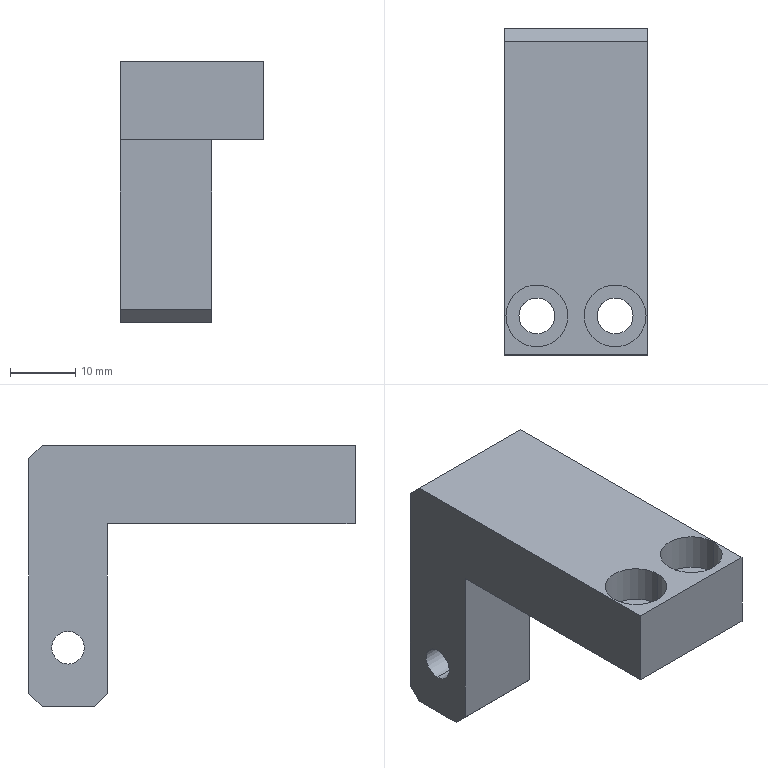Part | STEP file | PN_0018 Mount electronic clip limit block B | 1 solid | 25 faces | box 22 x 50 x 40 mm | volume 16406 mm3 | plane 15 | cylinder 10 | commonest cylinder face diameters 5.5 x4 9.5 x4 5 x2